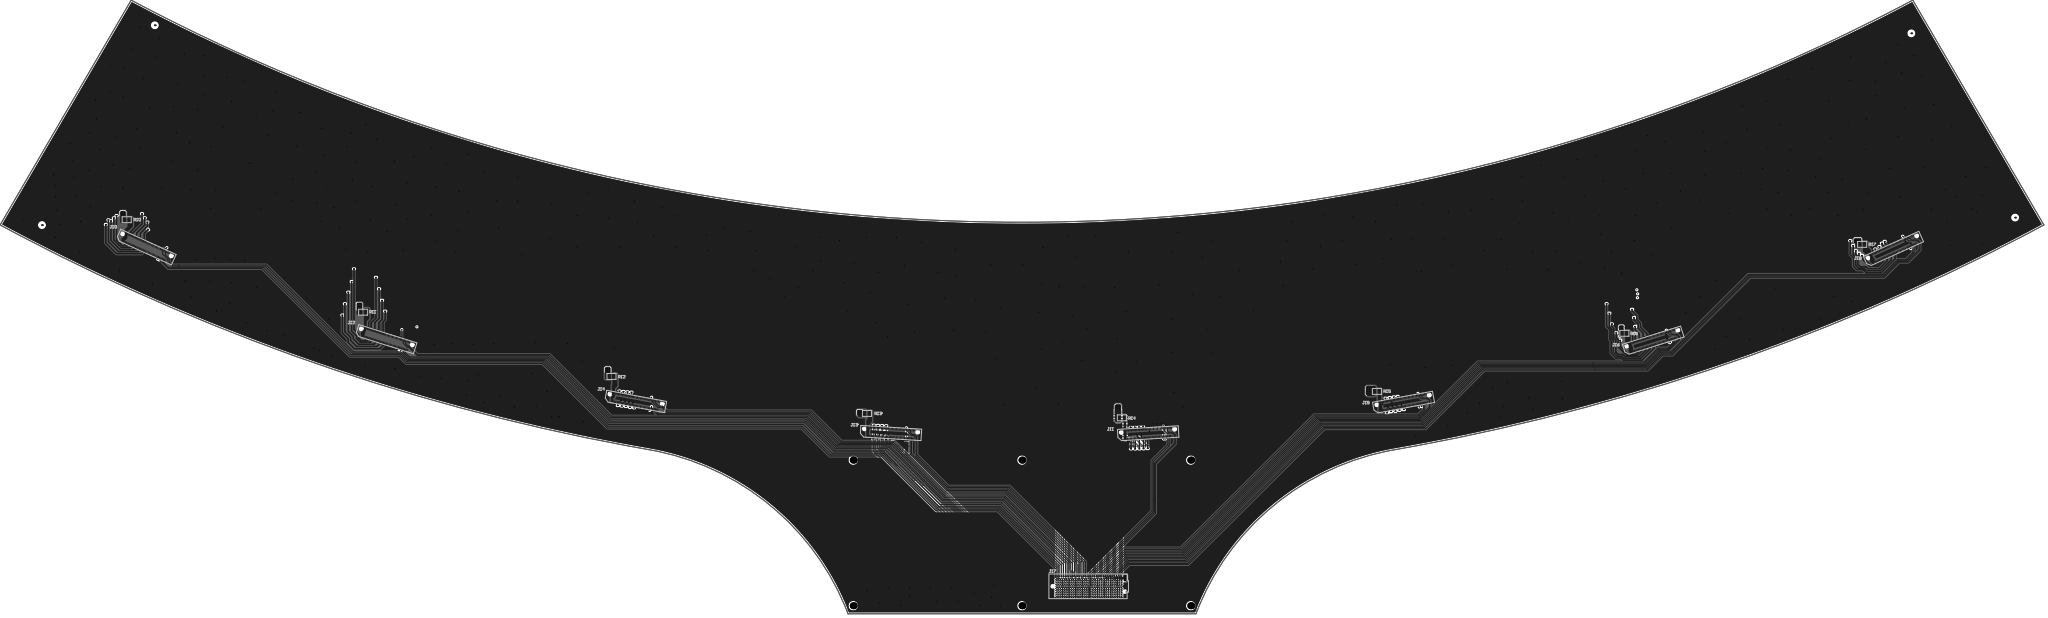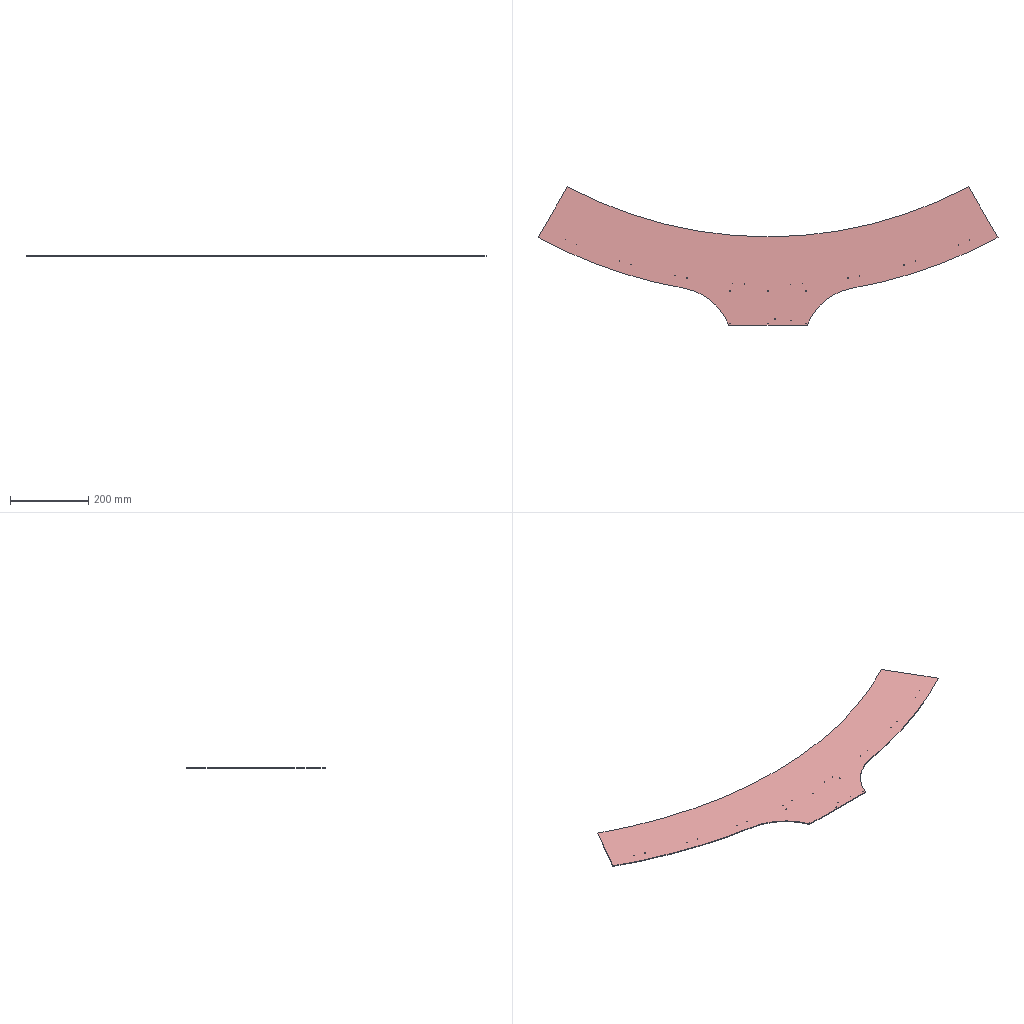Circuit board layout | Altium Designer | box 1175 x 354 x 1.8 mm
Layer stack:
# Altium Designer layer stack of  (unit mm; dielectric type: 0 none, 1 core, 2 prepreg, 3 surface material)
index,name,kind,layer,copper_thickness_mm,dielectric_type,dielectric_thickness_mm,dielectric_material,dielectric_constant
0,Top Paste,other,,,,,,
1,Top Overlay,other,,,,,,
2,Top Solder,dielectric,,,3,0.0102,Solder Resist,3.5
3,Top Layer,copper,Top Layer,0.0356,,,,
4,Dielectric1,dielectric,,,1,0.32,FR-4,4.8
5,GND2,copper,GND2,0.0356,,,,
6,Dielectric4,dielectric,,,2,0.32,FR-4,4.8
7,SIG3,copper,SIG3,0.0356,,,,
8,Dielectric3,dielectric,,,1,0.32,FR-4,4.8
9,SIG4,copper,SIG4,0.0356,,,,
10,Dielectric2,dielectric,,,2,0.32,FR-4,4.8
11,POWER5,copper,POWER5,0.0356,,,,
12,Dielectric5,dielectric,,,1,0.32,FR-4,4.8
13,Bottom Layer,copper,Bottom Layer,0.0356,,,,
14,Bottom Solder,dielectric,,,3,0.0102,Solder Resist,3.5
15,Bottom Overlay,other,,,,,,
16,Bottom Paste,other,,,,,,
# drill layer pairs: low layer,high layer
drill_pair,Top Layer,Bottom Layer
Part placement:
Designator,Comment,Layer,Footprint,Center-X(mm),Center-Y(mm),Rotation
R17,100R,TopLayer,R1210,1680.464,923.544,180
R16,100R,TopLayer,R1210,1543.812,872.236,180
R15,100R,TopLayer,R1210,1401.572,838.708,180
R14,100R,TopLayer,R1210,1254.989,823.493,180
R13,100R,TopLayer,R1210,1108.456,826.008,180
R12,100R,TopLayer,R1210,961.644,847.344,180
R11,100R,TopLayer,R1210,818.896,884.428,180
R10,100R,TopLayer,R1210,683.006,937.768,180
J12,ERF8-035-XX.X-X-DV,TopLayer,ERF8-035-XX.X-X-DV,832.557,868.846,162.43
J17,SEAF-30-XX.X-XX-10-X-A,TopLayer,SEAF-30-XX.X-XX-10-X-A,1236.037,726.283,0, 300 Pins"
J18,ERM8-035-XX.X-X-DV,TopLayer,ERF8-035-XX.X-X-DV,1697.845,920.852,204.43
J16,ERF8-035-XX.X-X-DV,TopLayer,ERF8-035-XX.X-X-DV,1559.924,867.996,197.43
J15,ERF8-035-XX.X-X-DV,TopLayer,ERF8-035-XX.X-X-DV,1416.6,832.395,190.43
J14,ERF8-035-XX.X-X-DV,TopLayer,ERF8-035-XX.X-X-DV,975.797,832.91,169.43
J13,ERF8-035-XX.X-X-DV,TopLayer,ERF8-035-XX.X-X-DV,1122.343,814.72,176.43
J11,ERF8-035-XX.X-X-DV,TopLayer,ERF8-035-XX.X-X-DV,1270.012,814.548,183.43
J10,ERF8-035-XX.X-X-DV,TopLayer,ERF8-035-XX.X-X-DV,694.758,922.025,155.43
Pad and via stacks:
# Altium Designer via and pad stacks of  (unit mm). Each distinct definition once, with the count of objects using it.
# via: kind,start_layer,end_layer,hole_mm,diameter_mm,mode(0 simple;1 top-mid-bottom;2 full stack),diameter_per_layer,count,example_net
# pad: kind,layer,hole_mm,hole_type(0 round;1 square;2 slot),plating,top_size,top_shape(1 round;2 rect;3 octagon;9 rounded rect),mid_size,bottom_size,mode,footprint,size_per_layer,count,example
pad,Multi-Layer,1.45,0,unplated,0x0,1,0x0,0x0,0,ERF8-035-XX.X-X-DV,,16,J13.MH2
pad,Multi-Layer,1.27,0,unplated,0x0,1,0x0,0x0,0,SEAF-30-XX.X-XX-10-X-A,,2,J17.MH2
pad,Multi-Layer,2.2,0,plated,4x4,1,4x4,4x4,0,,,6,0
pad,Top Layer,0,0,plated,1x1,1,1x1,1x1,0,,,4,0
pad,Top Layer,0,0,unplated,1.1x0.5,2,1.1x0.5,1.1x0.5,0,ERF8-035-XX.X-X-DV,,560,J13.61
pad,Top Layer,0,0,unplated,0.635x0.635,1,0.635x0.635,0.635x0.635,0,SEAF-30-XX.X-XX-10-X-A,,300,J17.K30
pad,Top Layer,0,0,plated,2.7x1.6,2,2.7x1.6,2.7x1.6,0,R1210,,16,R10.2
pad,Bottom Layer,0,0,plated,1x1,1,1x1,1x1,0,,,4,0
via,Top Layer,Bottom Layer,0.3048,0.6096,0,,684,DGND
via,Top Layer,Bottom Layer,0.2286,0.4572,0,,425,IO1_CH2
Copper pours:
name,layer,net,type(0 solid;1 hatched;2 none)
Top Layer-No Net,Top Layer,DGND,0
Top Layer-No Net,Top Layer,5V_POWERIN0,0
Top Layer-No Net,Top Layer,5V_POWERIN2,0
Top Layer-No Net,Top Layer,5V_POWERIN4,0
Top Layer-No Net,Top Layer,5V_OUT,0
Top Layer-No Net,Top Layer,5V_OUT,0
Top Layer-No Net,Top Layer,5V_OUT,0
Top Layer-No Net,Top Layer,5V_OUT,0
Top Layer-No Net,Top Layer,5V_OUT,0
Top Layer-No Net,Top Layer,5V_OUT,0
Top Layer-No Net,Top Layer,5V_OUT,0
Top Layer-No Net,Top Layer,5V_OUT,0
Top Layer-No Net,Top Layer,5V_OUT,0
Top Layer-No Net,Top Layer,5V_POWERIN1,0
Top Layer-No Net,Top Layer,5V_POWERIN3,0
Top Layer-No Net,Top Layer,5V_POWERIN5,0
Top Layer-No Net,Top Layer,5V_POWERIN6,0
Top Layer-No Net,Top Layer,5V_POWERIN7,0
Top Layer-No Net,SIG3,DGND,0
Top Layer-No Net,SIG4,DGND,0
Top Layer-No Net,Bottom Layer,DGND,0
Design rules, without the lines most boards share:
# Altium Designer design rules of  (exported by Altium Designer, unit mm)
# columns: name | kind | enabled | priority | scope1 | scope2 | descriptor | typed fields (field=value)
PolygonConnect_1 | 20 | enabled | 1 | isvia | All | Polygon Connect Rule(Direct Connect )(Conductor Width=10mil) (Relief Angle=90 Angle) (Entries=4) (Air Gap Width=10mil) (isvia),(All) | connect_style(0=relief,1=direct,2=none)=1 relief_conductor_width=0.254 relief_entries=4
Clearance | 0 | enabled | 1 | All | All | Clearance Constraint (Gap=5mil) (All),(All) | gap=0.127
PlaneConnect | 6 | enabled | 1 | All | All | Power Plane Connect Rule(Direct Connect )(Expansion=20mil) (Conductor Width=10mil) (Air Gap=10mil) (Entries=4) (All) | relief_conductor_width=0.254 relief_entries=4 relief_expansion=0.508
PolygonConnect | 20 | enabled | 2 | All | All | Polygon Connect Rule(Relief Connect )(Conductor Width=10mil) (Relief Angle=90 Angle) (Entries=4) (Air Gap Width=10mil) (All),(All) | connect_style(0=relief,1=direct,2=none)=0 relief_conductor_width=0.254 relief_entries=4
Width | 2 | enabled | 1 | All | All | Width Constraint (Min=5mil) (Max=20mil) (Preferred=5mil) (All) |
RoutingVias | 11 | enabled | 1 | All | All | Routing Via (MinHoleWidth=12mil) (MaxHoleWidth=12mil) (PreferredHoleWidth=12mil) (MinWidth=24mil) (MaxWidth=24mil) (PreferedWidth=24mil) (All) | via_min_hole=0.3048 via_max_hole=0.3048 via_preferred_diameter=0.6096 via_preferred_hole=0.3048
SolderMaskExpansion | 13 | enabled | 1 | All | All | Solder Mask Expansion (Expansion =4mil) (All) | expansion=0.1016
DiffPairsRouting | 51 | enabled | 1 | All | All | Differential Pairs Uncoupled Length using the Gap Constraints (Min=5mil) (Max=5mil) (Prefered=5mil)  and Width Constraints (Min=15mil) (Max=15mil) (Prefered=15mil) (All) |
HoleToHoleClearance | 52 | enabled | 1 | All | All | Hole To Hole Clearance (Gap=0mil) (All),(All) | gap=0
MinimumSolderMaskSliver | 53 | enabled | 1 | All | All | Minimum Solder Mask Sliver (Gap=0mil) (All),(All) |
SilkscreenOverComponentPads | 54 | enabled | 1 | IsPad | All | Silk To Solder Mask (Clearance=0mil) (IsPad),(All) |
SilkToSilkClearance | 55 | enabled | 1 | All | All | Silk to Silk (Clearance=0mil) (All),(All) |
Classes set for this board:
# Altium Designer classes of  (member kind: 0 net, 1 component, 2 from-to, 3 pad, 4 layer, 5 differential pair, 6 design channel, 7 polygon, 8 structure, 9 xSignal)
# columns: class name | member kind | superclass | members
BackPlane | 1 | no | J10; J11; J12; J13; J14; J15; J16; J17; J18; R10; R11; R12; R13; R14; R15; R16; R17; J12; R10; R11; R12; R13; R14; R15; R16; R17;